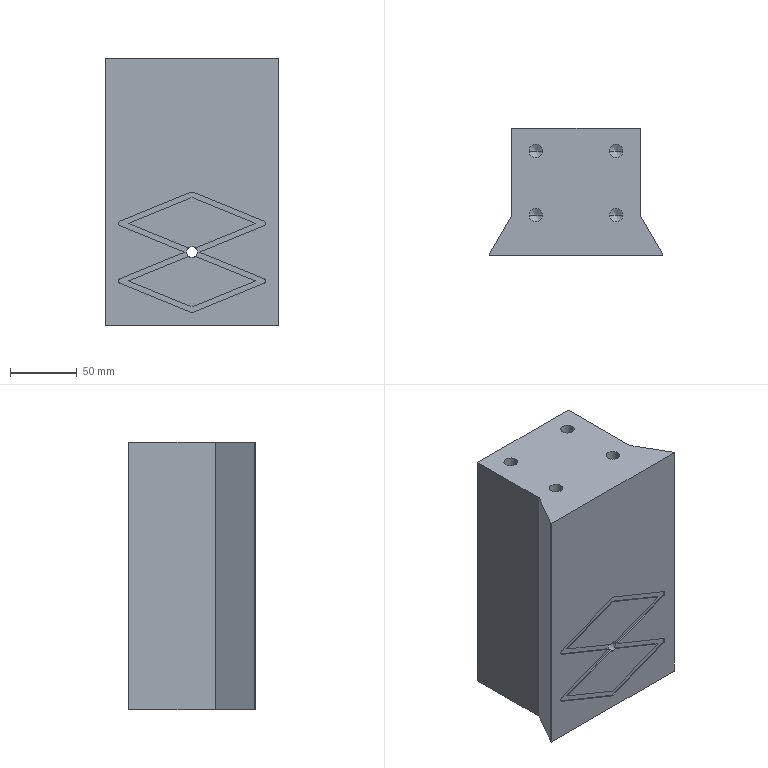Part | STEP file | DAU BUA | 1 solid | 74 faces | box 130 x 95 x 200 mm | volume 1902985 mm3 | plane 29 | cylinder 27 | cone 18 | commonest cylinder face diameters 8.376 x8 10.106 x8 4 x7 8 x2 15 x2